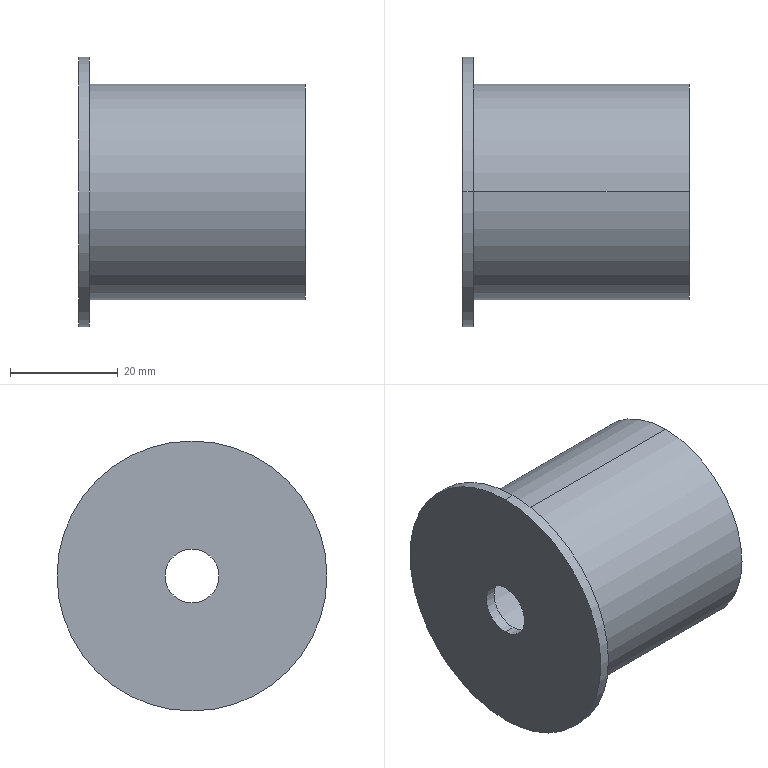Part | SolidWorks | features Revolution 1 | 1 solid | 12 faces | box 42 x 50 x 50 mm | volume 13320 mm3 | cylinder 8 | plane 4 | commonest cylinder face diameters 10 x2 36 x2 40 x2 50 x2
STEP:
#1=CARTESIAN_POINT('',(2.,0.,-5.));
#2=VERTEX_POINT('',#1);
#3=CARTESIAN_POINT('',(2.,0.,5.));
#4=VERTEX_POINT('',#3);
#5=CARTESIAN_POINT('',(2.,0.,0.));
#6=DIRECTION('',(-1.,0.,0.));
#7=DIRECTION('',(0.,0.,1.));
#8=AXIS2_PLACEMENT_3D('',#5,#6,#7);
#9=CIRCLE('',#8,5.);
#10=EDGE_CURVE('',#2,#4,#9,.T.);
#11=ORIENTED_EDGE('',*,*,#10,.F.);
#12=CARTESIAN_POINT('',(0.,0.,-5.));
#13=VERTEX_POINT('',#12);
#14=CARTESIAN_POINT('',(0.,0.,-5.));
#15=DIRECTION('',(-1.,0.,0.));
#16=VECTOR('',#15,1000.);
#17=LINE('',#14,#16);
#18=EDGE_CURVE('',#2,#13,#17,.T.);
#19=ORIENTED_EDGE('',*,*,#18,.T.);
#20=CARTESIAN_POINT('',(0.,0.,5.));
#21=VERTEX_POINT('',#20);
#22=CARTESIAN_POINT('',(0.,0.,0.));
#23=DIRECTION('',(-1.,0.,0.));
#24=DIRECTION('',(0.,0.,1.));
#25=AXIS2_PLACEMENT_3D('',#22,#23,#24);
#26=CIRCLE('',#25,5.);
#27=EDGE_CURVE('',#13,#21,#26,.T.);
#28=ORIENTED_EDGE('',*,*,#27,.T.);
#29=CARTESIAN_POINT('',(0.,0.,5.));
#30=DIRECTION('',(-1.,0.,0.));
#31=VECTOR('',#30,1000.);
#32=LINE('',#29,#31);
#33=EDGE_CURVE('',#4,#21,#32,.T.);
#34=ORIENTED_EDGE('',*,*,#33,.F.);
#35=EDGE_LOOP('',(#11,#19,#28,#34));
#36=FACE_OUTER_BOUND('',#35,.T.);
#37=CARTESIAN_POINT('',(0.,0.,0.));
#38=DIRECTION('',(-1.,0.,0.));
#39=DIRECTION('',(0.,0.,1.));
#40=AXIS2_PLACEMENT_3D('',#37,#38,#39);
#41=CYLINDRICAL_SURFACE('',#40,5.);
#42=ADVANCED_FACE('',(#36),#41,.F.);
#43=CARTESIAN_POINT('',(42.,0.,-18.));
#44=VERTEX_POINT('',#43);
#45=CARTESIAN_POINT('',(42.,0.,18.));
#46=VERTEX_POINT('',#45);
#47=CARTESIAN_POINT('',(42.,0.,0.));
#48=DIRECTION('',(-1.,0.,0.));
#49=DIRECTION('',(0.,0.,1.));
#50=AXIS2_PLACEMENT_3D('',#47,#48,#49);
#51=CIRCLE('',#50,18.);
#52=EDGE_CURVE('',#44,#46,#51,.T.);
#53=ORIENTED_EDGE('',*,*,#52,.F.);
#54=CARTESIAN_POINT('',(2.,0.,-18.));
#55=VERTEX_POINT('',#54);
#56=CARTESIAN_POINT('',(0.,0.,-18.));
#57=DIRECTION('',(-1.,0.,0.));
#58=VECTOR('',#57,1000.);
#59=LINE('',#56,#58);
#60=EDGE_CURVE('',#44,#55,#59,.T.);
#61=ORIENTED_EDGE('',*,*,#60,.T.);
#62=CARTESIAN_POINT('',(2.,0.,18.));
#63=VERTEX_POINT('',#62);
#64=CARTESIAN_POINT('',(2.,0.,0.));
#65=DIRECTION('',(-1.,0.,0.));
#66=DIRECTION('',(0.,0.,1.));
#67=AXIS2_PLACEMENT_3D('',#64,#65,#66);
#68=CIRCLE('',#67,18.);
#69=EDGE_CURVE('',#55,#63,#68,.T.);
#70=ORIENTED_EDGE('',*,*,#69,.T.);
#71=CARTESIAN_POINT('',(0.,0.,18.));
#72=DIRECTION('',(-1.,0.,0.));
#73=VECTOR('',#72,1000.);
#74=LINE('',#71,#73);
#75=EDGE_CURVE('',#46,#63,#74,.T.);
#76=ORIENTED_EDGE('',*,*,#75,.F.);
#77=EDGE_LOOP('',(#53,#61,#70,#76));
#78=FACE_OUTER_BOUND('',#77,.T.);
#79=CARTESIAN_POINT('',(0.,0.,0.));
#80=DIRECTION('',(-1.,0.,0.));
#81=DIRECTION('',(0.,0.,1.));
#82=AXIS2_PLACEMENT_3D('',#79,#80,#81);
#83=CYLINDRICAL_SURFACE('',#82,18.);
#84=ADVANCED_FACE('',(#78),#83,.F.);
#85=CARTESIAN_POINT('',(42.,0.,20.));
#86=VERTEX_POINT('',#85);
#87=CARTESIAN_POINT('',(42.,0.,-20.));
#88=VERTEX_POINT('',#87);
#89=CARTESIAN_POINT('',(42.,0.,0.));
#90=DIRECTION('',(-1.,0.,0.));
#91=DIRECTION('',(0.,0.,1.));
#92=AXIS2_PLACEMENT_3D('',#89,#90,#91);
#93=CIRCLE('',#92,20.);
#94=EDGE_CURVE('',#86,#88,#93,.T.);
#95=ORIENTED_EDGE('',*,*,#94,.T.);
#96=CARTESIAN_POINT('',(2.,0.,-20.));
#97=VERTEX_POINT('',#96);
#98=CARTESIAN_POINT('',(0.,0.,-20.));
#99=DIRECTION('',(-1.,0.,0.));
#100=VECTOR('',#99,1000.);
#101=LINE('',#98,#100);
#102=EDGE_CURVE('',#88,#97,#101,.T.);
#103=ORIENTED_EDGE('',*,*,#102,.T.);
#104=CARTESIAN_POINT('',(2.,0.,20.));
#105=VERTEX_POINT('',#104);
#106=CARTESIAN_POINT('',(2.,0.,0.));
#107=DIRECTION('',(-1.,0.,0.));
#108=DIRECTION('',(0.,0.,1.));
#109=AXIS2_PLACEMENT_3D('',#106,#107,#108);
#110=CIRCLE('',#109,20.);
#111=EDGE_CURVE('',#105,#97,#110,.T.);
#112=ORIENTED_EDGE('',*,*,#111,.F.);
#113=CARTESIAN_POINT('',(0.,0.,20.));
#114=DIRECTION('',(-1.,0.,0.));
#115=VECTOR('',#114,1000.);
#116=LINE('',#113,#115);
#117=EDGE_CURVE('',#86,#105,#116,.T.);
#118=ORIENTED_EDGE('',*,*,#117,.F.);
#119=EDGE_LOOP('',(#95,#103,#112,#118));
#120=FACE_OUTER_BOUND('',#119,.T.);
#121=CARTESIAN_POINT('',(0.,0.,0.));
#122=DIRECTION('',(-1.,0.,0.));
#123=DIRECTION('',(0.,0.,1.));
#124=AXIS2_PLACEMENT_3D('',#121,#122,#123);
#125=CYLINDRICAL_SURFACE('',#124,20.);
#126=ADVANCED_FACE('',(#120),#125,.T.);
#127=CARTESIAN_POINT('',(2.,0.,25.));
#128=VERTEX_POINT('',#127);
#129=CARTESIAN_POINT('',(2.,0.,-25.));
#130=VERTEX_POINT('',#129);
#131=CARTESIAN_POINT('',(2.,0.,0.));
#132=DIRECTION('',(-1.,0.,0.));
#133=DIRECTION('',(0.,0.,1.));
#134=AXIS2_PLACEMENT_3D('',#131,#132,#133);
#135=CIRCLE('',#134,25.);
#136=EDGE_CURVE('',#128,#130,#135,.T.);
#137=ORIENTED_EDGE('',*,*,#136,.T.);
#138=CARTESIAN_POINT('',(0.,0.,-25.));
#139=VERTEX_POINT('',#138);
#140=CARTESIAN_POINT('',(0.,0.,-25.));
#141=DIRECTION('',(-1.,0.,0.));
#142=VECTOR('',#141,1000.);
#143=LINE('',#140,#142);
#144=EDGE_CURVE('',#130,#139,#143,.T.);
#145=ORIENTED_EDGE('',*,*,#144,.T.);
#146=CARTESIAN_POINT('',(0.,0.,25.));
#147=VERTEX_POINT('',#146);
#148=CARTESIAN_POINT('',(0.,0.,0.));
#149=DIRECTION('',(-1.,0.,0.));
#150=DIRECTION('',(0.,0.,1.));
#151=AXIS2_PLACEMENT_3D('',#148,#149,#150);
#152=CIRCLE('',#151,25.);
#153=EDGE_CURVE('',#147,#139,#152,.T.);
#154=ORIENTED_EDGE('',*,*,#153,.F.);
#155=CARTESIAN_POINT('',(0.,0.,25.));
#156=DIRECTION('',(-1.,0.,0.));
#157=VECTOR('',#156,1000.);
#158=LINE('',#155,#157);
#159=EDGE_CURVE('',#128,#147,#158,.T.);
#160=ORIENTED_EDGE('',*,*,#159,.F.);
#161=EDGE_LOOP('',(#137,#145,#154,#160));
#162=FACE_OUTER_BOUND('',#161,.T.);
#163=CARTESIAN_POINT('',(0.,0.,0.));
#164=DIRECTION('',(-1.,0.,0.));
#165=DIRECTION('',(0.,0.,1.));
#166=AXIS2_PLACEMENT_3D('',#163,#164,#165);
#167=CYLINDRICAL_SURFACE('',#166,25.);
#168=ADVANCED_FACE('',(#162),#167,.T.);
#169=CARTESIAN_POINT('',(0.,0.,0.));
#170=DIRECTION('',(-1.,0.,0.));
#171=DIRECTION('',(0.,0.,1.));
#172=AXIS2_PLACEMENT_3D('',#169,#170,#171);
#173=CIRCLE('',#172,5.);
#174=EDGE_CURVE('',#21,#13,#173,.T.);
#175=ORIENTED_EDGE('',*,*,#174,.F.);
#176=ORIENTED_EDGE('',*,*,#27,.F.);
#177=EDGE_LOOP('',(#175,#176));
#178=FACE_BOUND('',#177,.T.);
#179=ORIENTED_EDGE('',*,*,#153,.T.);
#180=CARTESIAN_POINT('',(0.,0.,0.));
#181=DIRECTION('',(-1.,0.,0.));
#182=DIRECTION('',(0.,0.,1.));
#183=AXIS2_PLACEMENT_3D('',#180,#181,#182);
#184=CIRCLE('',#183,25.);
#185=EDGE_CURVE('',#139,#147,#184,.T.);
#186=ORIENTED_EDGE('',*,*,#185,.T.);
#187=EDGE_LOOP('',(#179,#186));
#188=FACE_OUTER_BOUND('',#187,.T.);
#189=CARTESIAN_POINT('',(0.,5.,0.));
#190=DIRECTION('',(1.,0.,0.));
#191=DIRECTION('',(0.,0.,-1.));
#192=AXIS2_PLACEMENT_3D('',#189,#190,#191);
#193=PLANE('',#192);
#194=ADVANCED_FACE('',(#178,#188),#193,.F.);
#195=ORIENTED_EDGE('',*,*,#144,.F.);
#196=CARTESIAN_POINT('',(2.,0.,0.));
#197=DIRECTION('',(-1.,0.,0.));
#198=DIRECTION('',(0.,0.,1.));
#199=AXIS2_PLACEMENT_3D('',#196,#197,#198);
#200=CIRCLE('',#199,25.);
#201=EDGE_CURVE('',#130,#128,#200,.T.);
#202=ORIENTED_EDGE('',*,*,#201,.T.);
#203=ORIENTED_EDGE('',*,*,#159,.T.);
#204=ORIENTED_EDGE('',*,*,#185,.F.);
#205=EDGE_LOOP('',(#195,#202,#203,#204));
#206=FACE_OUTER_BOUND('',#205,.T.);
#207=CARTESIAN_POINT('',(0.,0.,0.));
#208=DIRECTION('',(-1.,0.,0.));
#209=DIRECTION('',(0.,0.,1.));
#210=AXIS2_PLACEMENT_3D('',#207,#208,#209);
#211=CYLINDRICAL_SURFACE('',#210,25.);
#212=ADVANCED_FACE('',(#206),#211,.T.);
#213=ORIENTED_EDGE('',*,*,#136,.F.);
#214=ORIENTED_EDGE('',*,*,#201,.F.);
#215=EDGE_LOOP('',(#213,#214));
#216=FACE_OUTER_BOUND('',#215,.T.);
#217=ORIENTED_EDGE('',*,*,#111,.T.);
#218=CARTESIAN_POINT('',(2.,0.,0.));
#219=DIRECTION('',(-1.,0.,0.));
#220=DIRECTION('',(0.,0.,1.));
#221=AXIS2_PLACEMENT_3D('',#218,#219,#220);
#222=CIRCLE('',#221,20.);
#223=EDGE_CURVE('',#97,#105,#222,.T.);
#224=ORIENTED_EDGE('',*,*,#223,.T.);
#225=EDGE_LOOP('',(#217,#224));
#226=FACE_BOUND('',#225,.T.);
#227=CARTESIAN_POINT('',(2.,25.,0.));
#228=DIRECTION('',(-1.,0.,0.));
#229=DIRECTION('',(0.,0.,1.));
#230=AXIS2_PLACEMENT_3D('',#227,#228,#229);
#231=PLANE('',#230);
#232=ADVANCED_FACE('',(#216,#226),#231,.F.);
#233=ORIENTED_EDGE('',*,*,#102,.F.);
#234=CARTESIAN_POINT('',(42.,0.,0.));
#235=DIRECTION('',(-1.,0.,0.));
#236=DIRECTION('',(0.,0.,1.));
#237=AXIS2_PLACEMENT_3D('',#234,#235,#236);
#238=CIRCLE('',#237,20.);
#239=EDGE_CURVE('',#88,#86,#238,.T.);
#240=ORIENTED_EDGE('',*,*,#239,.T.);
#241=ORIENTED_EDGE('',*,*,#117,.T.);
#242=ORIENTED_EDGE('',*,*,#223,.F.);
#243=EDGE_LOOP('',(#233,#240,#241,#242));
#244=FACE_OUTER_BOUND('',#243,.T.);
#245=CARTESIAN_POINT('',(0.,0.,0.));
#246=DIRECTION('',(-1.,0.,0.));
#247=DIRECTION('',(0.,0.,1.));
#248=AXIS2_PLACEMENT_3D('',#245,#246,#247);
#249=CYLINDRICAL_SURFACE('',#248,20.);
#250=ADVANCED_FACE('',(#244),#249,.T.);
#251=ORIENTED_EDGE('',*,*,#94,.F.);
#252=ORIENTED_EDGE('',*,*,#239,.F.);
#253=EDGE_LOOP('',(#251,#252));
#254=FACE_OUTER_BOUND('',#253,.T.);
#255=CARTESIAN_POINT('',(42.,0.,0.));
#256=DIRECTION('',(-1.,0.,0.));
#257=DIRECTION('',(0.,0.,1.));
#258=AXIS2_PLACEMENT_3D('',#255,#256,#257);
#259=CIRCLE('',#258,18.);
#260=EDGE_CURVE('',#46,#44,#259,.T.);
#261=ORIENTED_EDGE('',*,*,#260,.T.);
#262=ORIENTED_EDGE('',*,*,#52,.T.);
#263=EDGE_LOOP('',(#261,#262));
#264=FACE_BOUND('',#263,.T.);
#265=CARTESIAN_POINT('',(42.,20.,0.));
#266=DIRECTION('',(-1.,0.,0.));
#267=DIRECTION('',(0.,0.,1.));
#268=AXIS2_PLACEMENT_3D('',#265,#266,#267);
#269=PLANE('',#268);
#270=ADVANCED_FACE('',(#254,#264),#269,.F.);
#271=ORIENTED_EDGE('',*,*,#60,.F.);
#272=ORIENTED_EDGE('',*,*,#260,.F.);
#273=ORIENTED_EDGE('',*,*,#75,.T.);
#274=CARTESIAN_POINT('',(2.,0.,0.));
#275=DIRECTION('',(-1.,0.,0.));
#276=DIRECTION('',(0.,0.,1.));
#277=AXIS2_PLACEMENT_3D('',#274,#275,#276);
#278=CIRCLE('',#277,18.);
#279=EDGE_CURVE('',#63,#55,#278,.T.);
#280=ORIENTED_EDGE('',*,*,#279,.T.);
#281=EDGE_LOOP('',(#271,#272,#273,#280));
#282=FACE_OUTER_BOUND('',#281,.T.);
#283=CARTESIAN_POINT('',(0.,0.,0.));
#284=DIRECTION('',(-1.,0.,0.));
#285=DIRECTION('',(0.,0.,1.));
#286=AXIS2_PLACEMENT_3D('',#283,#284,#285);
#287=CYLINDRICAL_SURFACE('',#286,18.);
#288=ADVANCED_FACE('',(#282),#287,.F.);
#289=ORIENTED_EDGE('',*,*,#279,.F.);
#290=ORIENTED_EDGE('',*,*,#69,.F.);
#291=EDGE_LOOP('',(#289,#290));
#292=FACE_OUTER_BOUND('',#291,.T.);
#293=CARTESIAN_POINT('',(2.,0.,0.));
#294=DIRECTION('',(-1.,0.,0.));
#295=DIRECTION('',(0.,0.,1.));
#296=AXIS2_PLACEMENT_3D('',#293,#294,#295);
#297=CIRCLE('',#296,5.);
#298=EDGE_CURVE('',#4,#2,#297,.T.);
#299=ORIENTED_EDGE('',*,*,#298,.T.);
#300=ORIENTED_EDGE('',*,*,#10,.T.);
#301=EDGE_LOOP('',(#299,#300));
#302=FACE_BOUND('',#301,.T.);
#303=CARTESIAN_POINT('',(2.,18.,0.));
#304=DIRECTION('',(-1.,0.,0.));
#305=DIRECTION('',(0.,0.,1.));
#306=AXIS2_PLACEMENT_3D('',#303,#304,#305);
#307=PLANE('',#306);
#308=ADVANCED_FACE('',(#292,#302),#307,.F.);
#309=ORIENTED_EDGE('',*,*,#18,.F.);
#310=ORIENTED_EDGE('',*,*,#298,.F.);
#311=ORIENTED_EDGE('',*,*,#33,.T.);
#312=ORIENTED_EDGE('',*,*,#174,.T.);
#313=EDGE_LOOP('',(#309,#310,#311,#312));
#314=FACE_OUTER_BOUND('',#313,.T.);
#315=CARTESIAN_POINT('',(0.,0.,0.));
#316=DIRECTION('',(-1.,0.,0.));
#317=DIRECTION('',(0.,0.,1.));
#318=AXIS2_PLACEMENT_3D('',#315,#316,#317);
#319=CYLINDRICAL_SURFACE('',#318,5.);
#320=ADVANCED_FACE('',(#314),#319,.F.);
#321=CLOSED_SHELL('',(#42,#84,#126,#168,#194,#212,#232,#250,#270,#288,#308,#320));
#322=MANIFOLD_SOLID_BREP('',#321);
#323=CARTESIAN_POINT('',(0.,0.,0.));
#324=DIRECTION('',(0.,0.,1.));
#325=DIRECTION('',(1.,0.,0.));
#326=AXIS2_PLACEMENT_3D('',#323,#324,#325);
#327=(LENGTH_UNIT()NAMED_UNIT(*)SI_UNIT(.MILLI.,.METRE.));
#328=UNCERTAINTY_MEASURE_WITH_UNIT(LENGTH_MEASURE(0.00001),#327,'','');
#329=(NAMED_UNIT(*)PLANE_ANGLE_UNIT()SI_UNIT($,.RADIAN.));
#330=(NAMED_UNIT(*)SI_UNIT($,.STERADIAN.)SOLID_ANGLE_UNIT());
#331=(GEOMETRIC_REPRESENTATION_CONTEXT(3)GLOBAL_UNCERTAINTY_ASSIGNED_CONTEXT((#328))GLOBAL_UNIT_ASSIGNED_CONTEXT((#327,#329,#330))REPRESENTATION_CONTEXT('',''));
#332=ADVANCED_BREP_SHAPE_REPRESENTATION('',(#322,#326),#331);